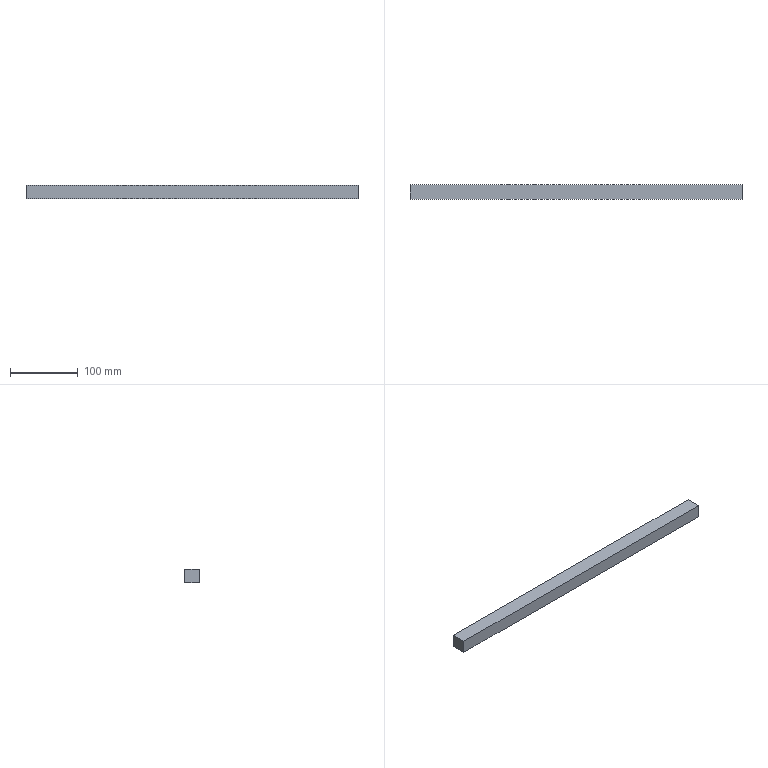Part | SolidWorks | features Extrusion 1 | 1 solid | 6 faces | box 490 x 22 x 20 mm | volume 215600 mm3 | plane 6
STEP:
#1=CARTESIAN_POINT('',(0.,22.,0.));
#2=VERTEX_POINT('',#1);
#3=CARTESIAN_POINT('',(0.,0.,0.));
#4=VERTEX_POINT('',#3);
#5=CARTESIAN_POINT('',(0.,0.,0.));
#6=DIRECTION('',(0.,-1.,0.));
#7=VECTOR('',#6,1000.);
#8=LINE('',#5,#7);
#9=EDGE_CURVE('',#2,#4,#8,.T.);
#10=ORIENTED_EDGE('',*,*,#9,.T.);
#11=CARTESIAN_POINT('',(0.,0.,20.));
#12=VERTEX_POINT('',#11);
#13=CARTESIAN_POINT('',(0.,0.,20.));
#14=DIRECTION('',(0.,0.,-1.));
#15=VECTOR('',#14,1000.);
#16=LINE('',#13,#15);
#17=EDGE_CURVE('',#12,#4,#16,.T.);
#18=ORIENTED_EDGE('',*,*,#17,.F.);
#19=CARTESIAN_POINT('',(0.,22.,20.));
#20=VERTEX_POINT('',#19);
#21=CARTESIAN_POINT('',(0.,0.,20.));
#22=DIRECTION('',(0.,-1.,0.));
#23=VECTOR('',#22,1000.);
#24=LINE('',#21,#23);
#25=EDGE_CURVE('',#20,#12,#24,.T.);
#26=ORIENTED_EDGE('',*,*,#25,.F.);
#27=CARTESIAN_POINT('',(0.,22.,20.));
#28=DIRECTION('',(0.,0.,-1.));
#29=VECTOR('',#28,1000.);
#30=LINE('',#27,#29);
#31=EDGE_CURVE('',#20,#2,#30,.T.);
#32=ORIENTED_EDGE('',*,*,#31,.T.);
#33=EDGE_LOOP('',(#10,#18,#26,#32));
#34=FACE_OUTER_BOUND('',#33,.T.);
#35=CARTESIAN_POINT('',(0.,0.,20.));
#36=DIRECTION('',(1.,0.,0.));
#37=DIRECTION('',(0.,0.,-1.));
#38=AXIS2_PLACEMENT_3D('',#35,#36,#37);
#39=PLANE('',#38);
#40=ADVANCED_FACE('',(#34),#39,.F.);
#41=CARTESIAN_POINT('',(490.,0.,0.));
#42=VERTEX_POINT('',#41);
#43=CARTESIAN_POINT('',(0.,0.,0.));
#44=DIRECTION('',(1.,0.,0.));
#45=VECTOR('',#44,1000.);
#46=LINE('',#43,#45);
#47=EDGE_CURVE('',#4,#42,#46,.T.);
#48=ORIENTED_EDGE('',*,*,#47,.T.);
#49=CARTESIAN_POINT('',(490.,0.,20.));
#50=VERTEX_POINT('',#49);
#51=CARTESIAN_POINT('',(490.,0.,20.));
#52=DIRECTION('',(0.,0.,-1.));
#53=VECTOR('',#52,1000.);
#54=LINE('',#51,#53);
#55=EDGE_CURVE('',#50,#42,#54,.T.);
#56=ORIENTED_EDGE('',*,*,#55,.F.);
#57=CARTESIAN_POINT('',(0.,0.,20.));
#58=DIRECTION('',(1.,0.,0.));
#59=VECTOR('',#58,1000.);
#60=LINE('',#57,#59);
#61=EDGE_CURVE('',#12,#50,#60,.T.);
#62=ORIENTED_EDGE('',*,*,#61,.F.);
#63=ORIENTED_EDGE('',*,*,#17,.T.);
#64=EDGE_LOOP('',(#48,#56,#62,#63));
#65=FACE_OUTER_BOUND('',#64,.T.);
#66=CARTESIAN_POINT('',(0.,0.,20.));
#67=DIRECTION('',(0.,1.,0.));
#68=DIRECTION('',(0.,0.,1.));
#69=AXIS2_PLACEMENT_3D('',#66,#67,#68);
#70=PLANE('',#69);
#71=ADVANCED_FACE('',(#65),#70,.F.);
#72=CARTESIAN_POINT('',(490.,22.,0.));
#73=VERTEX_POINT('',#72);
#74=CARTESIAN_POINT('',(490.,0.,0.));
#75=DIRECTION('',(0.,1.,0.));
#76=VECTOR('',#75,1000.);
#77=LINE('',#74,#76);
#78=EDGE_CURVE('',#42,#73,#77,.T.);
#79=ORIENTED_EDGE('',*,*,#78,.T.);
#80=CARTESIAN_POINT('',(490.,22.,20.));
#81=VERTEX_POINT('',#80);
#82=CARTESIAN_POINT('',(490.,22.,20.));
#83=DIRECTION('',(0.,0.,-1.));
#84=VECTOR('',#83,1000.);
#85=LINE('',#82,#84);
#86=EDGE_CURVE('',#81,#73,#85,.T.);
#87=ORIENTED_EDGE('',*,*,#86,.F.);
#88=CARTESIAN_POINT('',(490.,0.,20.));
#89=DIRECTION('',(0.,1.,0.));
#90=VECTOR('',#89,1000.);
#91=LINE('',#88,#90);
#92=EDGE_CURVE('',#50,#81,#91,.T.);
#93=ORIENTED_EDGE('',*,*,#92,.F.);
#94=ORIENTED_EDGE('',*,*,#55,.T.);
#95=EDGE_LOOP('',(#79,#87,#93,#94));
#96=FACE_OUTER_BOUND('',#95,.T.);
#97=CARTESIAN_POINT('',(490.,0.,20.));
#98=DIRECTION('',(-1.,0.,0.));
#99=DIRECTION('',(0.,0.,1.));
#100=AXIS2_PLACEMENT_3D('',#97,#98,#99);
#101=PLANE('',#100);
#102=ADVANCED_FACE('',(#96),#101,.F.);
#103=CARTESIAN_POINT('',(0.,22.,0.));
#104=DIRECTION('',(-1.,0.,0.));
#105=VECTOR('',#104,1000.);
#106=LINE('',#103,#105);
#107=EDGE_CURVE('',#73,#2,#106,.T.);
#108=ORIENTED_EDGE('',*,*,#107,.T.);
#109=ORIENTED_EDGE('',*,*,#31,.F.);
#110=CARTESIAN_POINT('',(0.,22.,20.));
#111=DIRECTION('',(-1.,0.,0.));
#112=VECTOR('',#111,1000.);
#113=LINE('',#110,#112);
#114=EDGE_CURVE('',#81,#20,#113,.T.);
#115=ORIENTED_EDGE('',*,*,#114,.F.);
#116=ORIENTED_EDGE('',*,*,#86,.T.);
#117=EDGE_LOOP('',(#108,#109,#115,#116));
#118=FACE_OUTER_BOUND('',#117,.T.);
#119=CARTESIAN_POINT('',(0.,22.,20.));
#120=DIRECTION('',(0.,-1.,0.));
#121=DIRECTION('',(0.,0.,-1.));
#122=AXIS2_PLACEMENT_3D('',#119,#120,#121);
#123=PLANE('',#122);
#124=ADVANCED_FACE('',(#118),#123,.F.);
#125=ORIENTED_EDGE('',*,*,#25,.T.);
#126=ORIENTED_EDGE('',*,*,#61,.T.);
#127=ORIENTED_EDGE('',*,*,#92,.T.);
#128=ORIENTED_EDGE('',*,*,#114,.T.);
#129=EDGE_LOOP('',(#125,#126,#127,#128));
#130=FACE_OUTER_BOUND('',#129,.T.);
#131=CARTESIAN_POINT('',(0.,0.,20.));
#132=DIRECTION('',(0.,0.,-1.));
#133=DIRECTION('',(-1.,0.,0.));
#134=AXIS2_PLACEMENT_3D('',#131,#132,#133);
#135=PLANE('',#134);
#136=ADVANCED_FACE('',(#130),#135,.F.);
#137=ORIENTED_EDGE('',*,*,#9,.F.);
#138=ORIENTED_EDGE('',*,*,#107,.F.);
#139=ORIENTED_EDGE('',*,*,#78,.F.);
#140=ORIENTED_EDGE('',*,*,#47,.F.);
#141=EDGE_LOOP('',(#137,#138,#139,#140));
#142=FACE_OUTER_BOUND('',#141,.T.);
#143=CARTESIAN_POINT('',(0.,0.,0.));
#144=DIRECTION('',(0.,0.,-1.));
#145=DIRECTION('',(-1.,0.,0.));
#146=AXIS2_PLACEMENT_3D('',#143,#144,#145);
#147=PLANE('',#146);
#148=ADVANCED_FACE('',(#142),#147,.T.);
#149=CLOSED_SHELL('',(#40,#71,#102,#124,#136,#148));
#150=MANIFOLD_SOLID_BREP('',#149);
#151=CARTESIAN_POINT('',(0.,0.,0.));
#152=DIRECTION('',(0.,0.,1.));
#153=DIRECTION('',(1.,0.,0.));
#154=AXIS2_PLACEMENT_3D('',#151,#152,#153);
#155=(LENGTH_UNIT()NAMED_UNIT(*)SI_UNIT(.MILLI.,.METRE.));
#156=UNCERTAINTY_MEASURE_WITH_UNIT(LENGTH_MEASURE(0.00001),#155,'','');
#157=(NAMED_UNIT(*)PLANE_ANGLE_UNIT()SI_UNIT($,.RADIAN.));
#158=(NAMED_UNIT(*)SI_UNIT($,.STERADIAN.)SOLID_ANGLE_UNIT());
#159=(GEOMETRIC_REPRESENTATION_CONTEXT(3)GLOBAL_UNCERTAINTY_ASSIGNED_CONTEXT((#156))GLOBAL_UNIT_ASSIGNED_CONTEXT((#155,#157,#158))REPRESENTATION_CONTEXT('',''));
#160=ADVANCED_BREP_SHAPE_REPRESENTATION('',(#150,#154),#159);